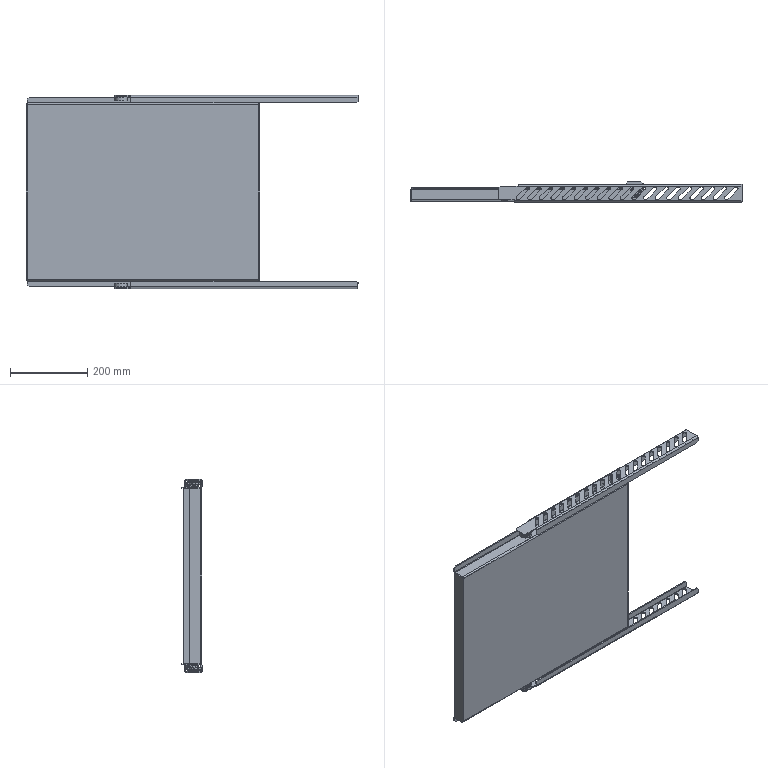Part | SolidWorks | 9 solids | 918 faces | box 859.852 x 52 x 499.996 mm | volume 1351190 mm3 | sphere 352 | plane 224 | cylinder 214 | torus 128 | commonest cylinder face diameters 10 x114 12 x16 8 x12 2 x8 13 x8 16.05 x8